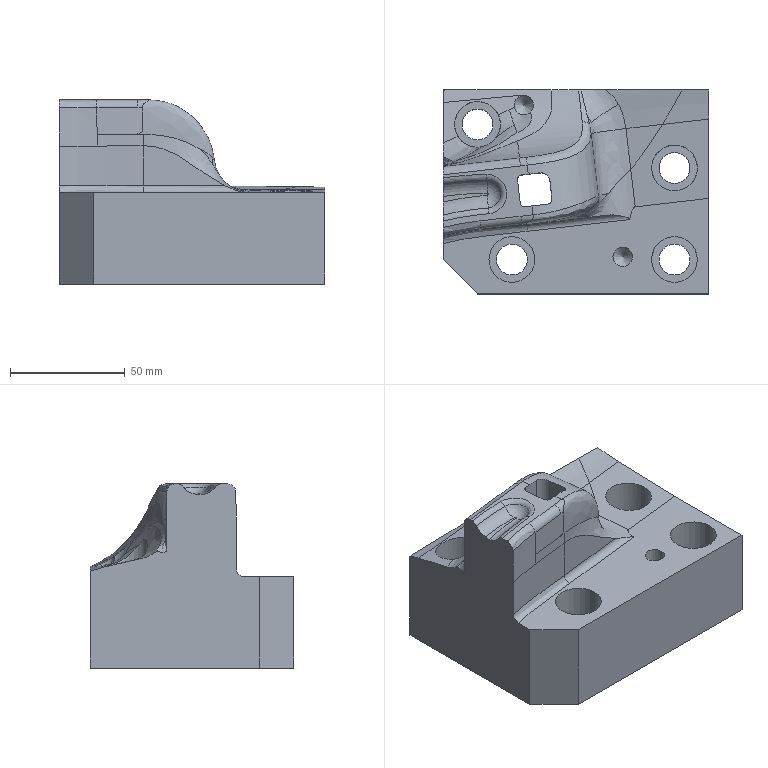Part | NX | features 23 2 | 1 solid | 96 faces | box 116 x 89.001 x 80.425 mm | volume 441156 mm3 | plane 34 | cylinder 27 | spline 26 | torus 7 | cone 2 | commonest cylinder face diameters 8 x5 13.5 x4 15 x4 20 x4 4 x3 7 x2